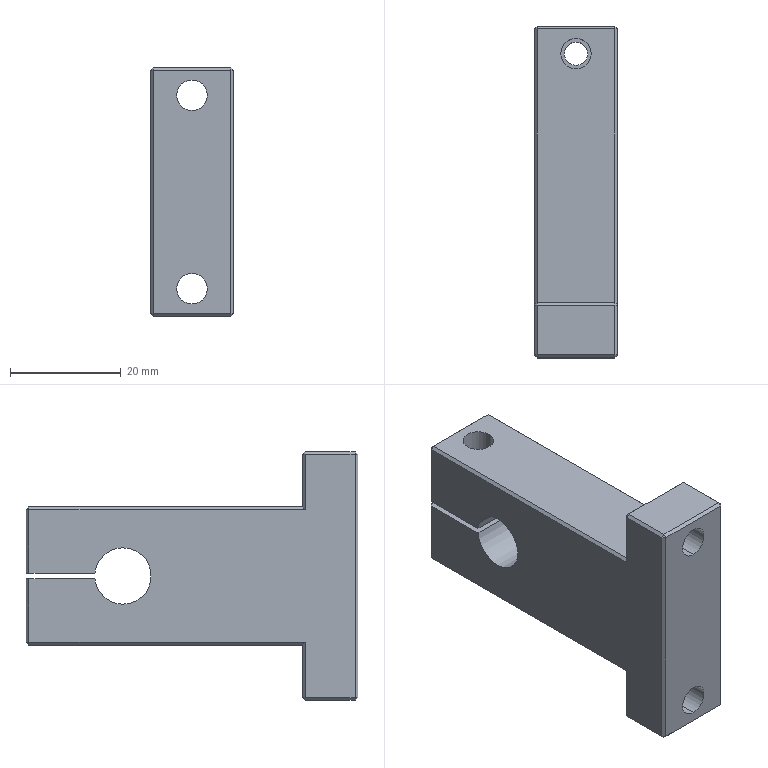Part | STEP file | 06-17 Screw locking block | 1 solid | 58 faces | box 15 x 60 x 45 mm | volume 23099 mm3 | plane 49 | cylinder 9 | commonest cylinder face diameters 5.5 x6 4.2 x2 10.2 x1